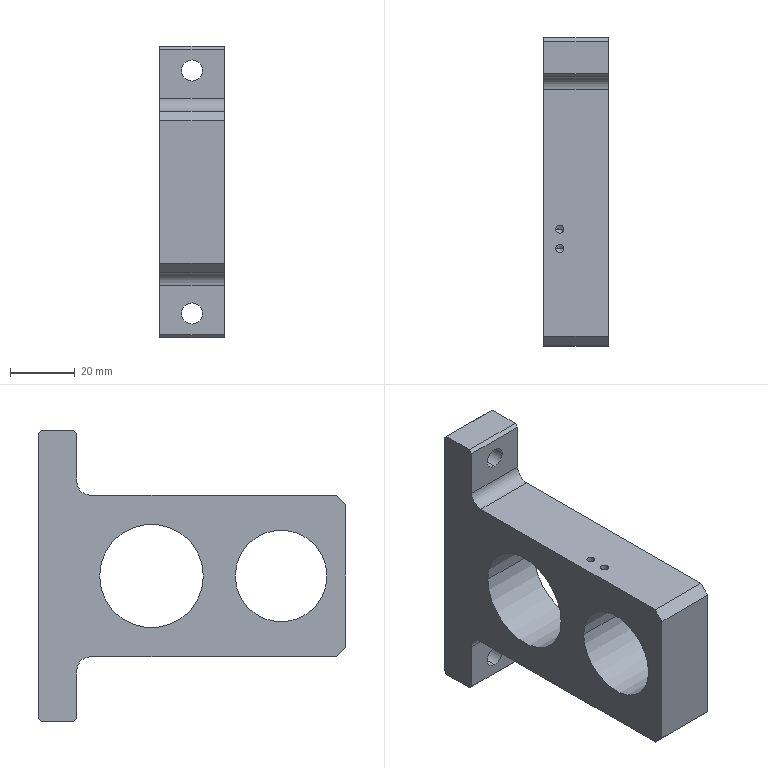Part | STEP file | Movable support plate_sand-blasted, oxidised | 1 solid | 82 faces | box 20 x 95 x 90 mm | volume 73168 mm3 | cylinder 38 | cone 28 | plane 16 | commonest cylinder face diameters 4.2 x20 2.5 x8 6.5 x4 8 x2 28.3 x2 32 x2